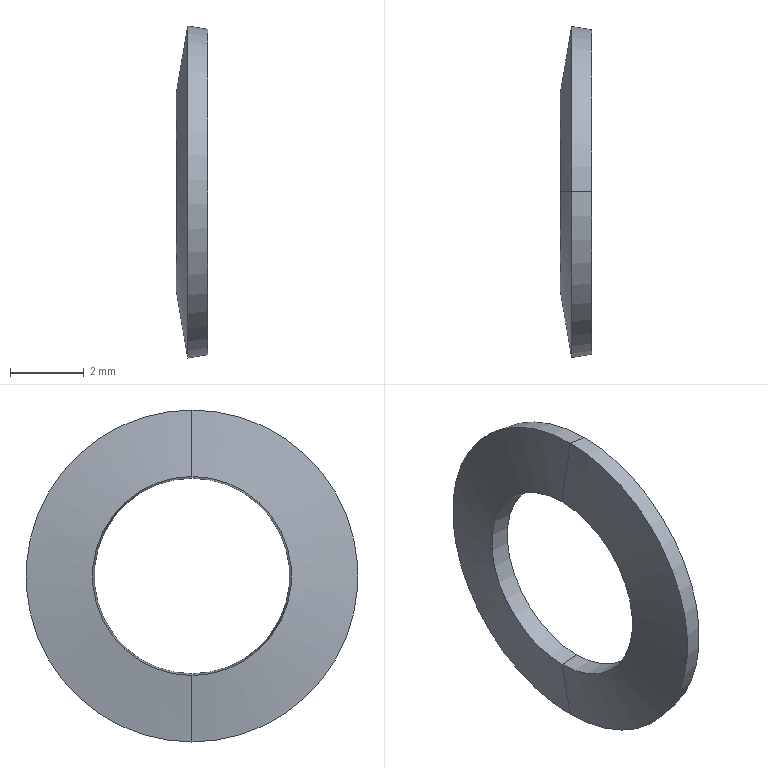Part | STEP file | CW5_Default | 1 solid | 8 faces | box 0.85 x 9 x 9 mm | volume 22.263 mm3 | cone 8
STEP:
#1=CARTESIAN_POINT('',(0.,0.,0.));
#2=DIRECTION('',(0.,0.,1.));
#3=DIRECTION('',(1.,0.,0.));
#4=AXIS2_PLACEMENT_3D('',#1,#2,#3);
#5=CARTESIAN_POINT('',(0.55,0.,2.65));
#6=VERTEX_POINT('',#5);
#7=CARTESIAN_POINT('',(0.,0.,2.697));
#8=VERTEX_POINT('',#7);
#9=CARTESIAN_POINT('',(0.,0.,2.697));
#10=DIRECTION('',(-0.9964,0.,0.08432));
#11=VECTOR('',#10,1.);
#12=LINE('',#9,#11);
#13=CARTESIAN_POINT('',(0.,0.,0.));
#14=DIRECTION('',(-1.,0.,0.));
#15=DIRECTION('',(0.,0.,1.));
#16=AXIS2_PLACEMENT_3D('',#13,#14,#15);
#17=CONICAL_SURFACE('',#16,2.697,0.08442);
#18=CARTESIAN_POINT('',(6.283,0.));
#19=DIRECTION('',(0.,1.));
#20=VECTOR('',#19,1.);
#21=LINE('',#18,#20);
#22=(GEOMETRIC_REPRESENTATION_CONTEXT(2)PARAMETRIC_REPRESENTATION_CONTEXT()REPRESENTATION_CONTEXT('',''));
#23=DEFINITIONAL_REPRESENTATION('',(#21),#22);
#24=PCURVE('',#17,#23);
#25=CARTESIAN_POINT('',(0.,0.,0.));
#26=DIRECTION('',(-1.,0.,0.));
#27=DIRECTION('',(0.,0.,1.));
#28=AXIS2_PLACEMENT_3D('',#25,#26,#27);
#29=CONICAL_SURFACE('',#28,2.697,0.08442);
#30=CARTESIAN_POINT('',(0.,0.));
#31=DIRECTION('',(0.,1.));
#32=VECTOR('',#31,1.);
#33=LINE('',#30,#32);
#34=(GEOMETRIC_REPRESENTATION_CONTEXT(2)PARAMETRIC_REPRESENTATION_CONTEXT()REPRESENTATION_CONTEXT('',''));
#35=DEFINITIONAL_REPRESENTATION('',(#33),#34);
#36=PCURVE('',#29,#35);
#37=SURFACE_CURVE('',#12,(#24,#36),.PCURVE_S1.);
#38=EDGE_CURVE('',#6,#8,#37,.T.);
#39=ORIENTED_EDGE('',*,*,#38,.T.);
#40=CARTESIAN_POINT('',(0.,0.,-2.697));
#41=VERTEX_POINT('',#40);
#42=CARTESIAN_POINT('',(0.,0.,0.));
#43=DIRECTION('',(-1.,0.,0.));
#44=DIRECTION('',(0.,0.,1.));
#45=AXIS2_PLACEMENT_3D('',#42,#43,#44);
#46=CIRCLE('',#45,2.697);
#47=CARTESIAN_POINT('',(0.,0.));
#48=DIRECTION('',(1.,0.));
#49=VECTOR('',#48,1.);
#50=LINE('',#47,#49);
#51=(GEOMETRIC_REPRESENTATION_CONTEXT(2)PARAMETRIC_REPRESENTATION_CONTEXT()REPRESENTATION_CONTEXT('',''));
#52=DEFINITIONAL_REPRESENTATION('',(#50),#51);
#53=PCURVE('',#17,#52);
#54=CARTESIAN_POINT('',(0.3074,0.,0.));
#55=DIRECTION('',(1.,0.,0.));
#56=DIRECTION('',(0.,0.,-1.));
#57=AXIS2_PLACEMENT_3D('',#54,#55,#56);
#58=CONICAL_SURFACE('',#57,4.5,1.402);
#59=CARTESIAN_POINT('',(9.425,-0.3074));
#60=DIRECTION('',(-1.,0.));
#61=VECTOR('',#60,1.);
#62=LINE('',#59,#61);
#63=(GEOMETRIC_REPRESENTATION_CONTEXT(2)PARAMETRIC_REPRESENTATION_CONTEXT()REPRESENTATION_CONTEXT('',''));
#64=DEFINITIONAL_REPRESENTATION('',(#62),#63);
#65=PCURVE('',#58,#64);
#66=SURFACE_CURVE('',#46,(#53,#65),.PCURVE_S1.);
#67=EDGE_CURVE('',#41,#8,#66,.T.);
#68=ORIENTED_EDGE('',*,*,#67,.F.);
#69=CARTESIAN_POINT('',(0.55,0.,-2.65));
#70=VERTEX_POINT('',#69);
#71=CARTESIAN_POINT('',(0.,0.,-2.697));
#72=DIRECTION('',(-0.9964,0.,-0.08432));
#73=VECTOR('',#72,1.);
#74=LINE('',#71,#73);
#75=CARTESIAN_POINT('',(3.142,0.));
#76=DIRECTION('',(0.,1.));
#77=VECTOR('',#76,1.);
#78=LINE('',#75,#77);
#79=(GEOMETRIC_REPRESENTATION_CONTEXT(2)PARAMETRIC_REPRESENTATION_CONTEXT()REPRESENTATION_CONTEXT('',''));
#80=DEFINITIONAL_REPRESENTATION('',(#78),#79);
#81=PCURVE('',#17,#80);
#82=CARTESIAN_POINT('',(3.142,0.));
#83=DIRECTION('',(0.,1.));
#84=VECTOR('',#83,1.);
#85=LINE('',#82,#84);
#86=(GEOMETRIC_REPRESENTATION_CONTEXT(2)PARAMETRIC_REPRESENTATION_CONTEXT()REPRESENTATION_CONTEXT('',''));
#87=DEFINITIONAL_REPRESENTATION('',(#85),#86);
#88=PCURVE('',#29,#87);
#89=SURFACE_CURVE('',#74,(#81,#88),.PCURVE_S1.);
#90=EDGE_CURVE('',#70,#41,#89,.T.);
#91=ORIENTED_EDGE('',*,*,#90,.F.);
#92=CARTESIAN_POINT('',(0.55,0.,0.));
#93=DIRECTION('',(-1.,0.,0.));
#94=DIRECTION('',(0.,0.,1.));
#95=AXIS2_PLACEMENT_3D('',#92,#93,#94);
#96=CIRCLE('',#95,2.65);
#97=CARTESIAN_POINT('',(0.,-0.55));
#98=DIRECTION('',(1.,0.));
#99=VECTOR('',#98,1.);
#100=LINE('',#97,#99);
#101=(GEOMETRIC_REPRESENTATION_CONTEXT(2)PARAMETRIC_REPRESENTATION_CONTEXT()REPRESENTATION_CONTEXT('',''));
#102=DEFINITIONAL_REPRESENTATION('',(#100),#101);
#103=PCURVE('',#17,#102);
#104=CARTESIAN_POINT('',(0.55,0.,0.));
#105=DIRECTION('',(1.,0.,0.));
#106=DIRECTION('',(0.,0.,-1.));
#107=AXIS2_PLACEMENT_3D('',#104,#105,#106);
#108=CONICAL_SURFACE('',#107,2.65,1.402);
#109=CARTESIAN_POINT('',(9.425,0.));
#110=DIRECTION('',(-1.,0.));
#111=VECTOR('',#110,1.);
#112=LINE('',#109,#111);
#113=(GEOMETRIC_REPRESENTATION_CONTEXT(2)PARAMETRIC_REPRESENTATION_CONTEXT()REPRESENTATION_CONTEXT('',''));
#114=DEFINITIONAL_REPRESENTATION('',(#112),#113);
#115=PCURVE('',#108,#114);
#116=SURFACE_CURVE('',#96,(#103,#115),.PCURVE_S1.);
#117=EDGE_CURVE('',#70,#6,#116,.T.);
#118=ORIENTED_EDGE('',*,*,#117,.T.);
#119=EDGE_LOOP('',(#39,#68,#91,#118));
#120=FACE_BOUND('',#119,.F.);
#121=ADVANCED_FACE('',(#120),#17,.F.);
#122=CARTESIAN_POINT('',(0.85,0.,-4.41));
#123=VERTEX_POINT('',#122);
#124=CARTESIAN_POINT('',(0.55,0.,-2.65));
#125=DIRECTION('',(0.168,0.,-0.9858));
#126=VECTOR('',#125,1.);
#127=LINE('',#124,#126);
#128=CARTESIAN_POINT('',(6.283,0.));
#129=DIRECTION('',(0.,1.));
#130=VECTOR('',#129,1.);
#131=LINE('',#128,#130);
#132=(GEOMETRIC_REPRESENTATION_CONTEXT(2)PARAMETRIC_REPRESENTATION_CONTEXT()REPRESENTATION_CONTEXT('',''));
#133=DEFINITIONAL_REPRESENTATION('',(#131),#132);
#134=PCURVE('',#108,#133);
#135=CARTESIAN_POINT('',(0.55,0.,0.));
#136=DIRECTION('',(1.,0.,0.));
#137=DIRECTION('',(0.,0.,-1.));
#138=AXIS2_PLACEMENT_3D('',#135,#136,#137);
#139=CONICAL_SURFACE('',#138,2.65,1.402);
#140=CARTESIAN_POINT('',(0.,0.));
#141=DIRECTION('',(0.,1.));
#142=VECTOR('',#141,1.);
#143=LINE('',#140,#142);
#144=(GEOMETRIC_REPRESENTATION_CONTEXT(2)PARAMETRIC_REPRESENTATION_CONTEXT()REPRESENTATION_CONTEXT('',''));
#145=DEFINITIONAL_REPRESENTATION('',(#143),#144);
#146=PCURVE('',#139,#145);
#147=SURFACE_CURVE('',#127,(#134,#146),.PCURVE_S1.);
#148=EDGE_CURVE('',#70,#123,#147,.T.);
#149=ORIENTED_EDGE('',*,*,#148,.T.);
#150=CARTESIAN_POINT('',(0.85,0.,4.41));
#151=VERTEX_POINT('',#150);
#152=CARTESIAN_POINT('',(0.85,0.,0.));
#153=DIRECTION('',(-1.,0.,0.));
#154=DIRECTION('',(0.,0.,1.));
#155=AXIS2_PLACEMENT_3D('',#152,#153,#154);
#156=CIRCLE('',#155,4.41);
#157=CARTESIAN_POINT('',(9.425,0.3));
#158=DIRECTION('',(-1.,0.));
#159=VECTOR('',#158,1.);
#160=LINE('',#157,#159);
#161=(GEOMETRIC_REPRESENTATION_CONTEXT(2)PARAMETRIC_REPRESENTATION_CONTEXT()REPRESENTATION_CONTEXT('',''));
#162=DEFINITIONAL_REPRESENTATION('',(#160),#161);
#163=PCURVE('',#108,#162);
#164=CARTESIAN_POINT('',(0.85,0.,0.));
#165=DIRECTION('',(-1.,0.,0.));
#166=DIRECTION('',(0.,0.,1.));
#167=AXIS2_PLACEMENT_3D('',#164,#165,#166);
#168=CONICAL_SURFACE('',#167,4.41,0.1644);
#169=CARTESIAN_POINT('',(0.,0.));
#170=DIRECTION('',(1.,0.));
#171=VECTOR('',#170,1.);
#172=LINE('',#169,#171);
#173=(GEOMETRIC_REPRESENTATION_CONTEXT(2)PARAMETRIC_REPRESENTATION_CONTEXT()REPRESENTATION_CONTEXT('',''));
#174=DEFINITIONAL_REPRESENTATION('',(#172),#173);
#175=PCURVE('',#168,#174);
#176=SURFACE_CURVE('',#156,(#163,#175),.PCURVE_S1.);
#177=EDGE_CURVE('',#123,#151,#176,.T.);
#178=ORIENTED_EDGE('',*,*,#177,.T.);
#179=CARTESIAN_POINT('',(0.55,0.,2.65));
#180=DIRECTION('',(0.168,0.,0.9858));
#181=VECTOR('',#180,1.);
#182=LINE('',#179,#181);
#183=CARTESIAN_POINT('',(3.142,0.));
#184=DIRECTION('',(0.,1.));
#185=VECTOR('',#184,1.);
#186=LINE('',#183,#185);
#187=(GEOMETRIC_REPRESENTATION_CONTEXT(2)PARAMETRIC_REPRESENTATION_CONTEXT()REPRESENTATION_CONTEXT('',''));
#188=DEFINITIONAL_REPRESENTATION('',(#186),#187);
#189=PCURVE('',#108,#188);
#190=CARTESIAN_POINT('',(3.142,0.));
#191=DIRECTION('',(0.,1.));
#192=VECTOR('',#191,1.);
#193=LINE('',#190,#192);
#194=(GEOMETRIC_REPRESENTATION_CONTEXT(2)PARAMETRIC_REPRESENTATION_CONTEXT()REPRESENTATION_CONTEXT('',''));
#195=DEFINITIONAL_REPRESENTATION('',(#193),#194);
#196=PCURVE('',#139,#195);
#197=SURFACE_CURVE('',#182,(#189,#196),.PCURVE_S1.);
#198=EDGE_CURVE('',#6,#151,#197,.T.);
#199=ORIENTED_EDGE('',*,*,#198,.F.);
#200=ORIENTED_EDGE('',*,*,#117,.F.);
#201=EDGE_LOOP('',(#149,#178,#199,#200));
#202=FACE_BOUND('',#201,.F.);
#203=ADVANCED_FACE('',(#202),#108,.F.);
#204=CARTESIAN_POINT('',(0.85,0.,0.));
#205=DIRECTION('',(-1.,0.,0.));
#206=DIRECTION('',(0.,0.,1.));
#207=AXIS2_PLACEMENT_3D('',#204,#205,#206);
#208=CIRCLE('',#207,4.41);
#209=CARTESIAN_POINT('',(0.85,0.,0.));
#210=DIRECTION('',(-1.,0.,0.));
#211=DIRECTION('',(0.,0.,1.));
#212=AXIS2_PLACEMENT_3D('',#209,#210,#211);
#213=CONICAL_SURFACE('',#212,4.41,0.1644);
#214=CARTESIAN_POINT('',(0.,0.));
#215=DIRECTION('',(1.,0.));
#216=VECTOR('',#215,1.);
#217=LINE('',#214,#216);
#218=(GEOMETRIC_REPRESENTATION_CONTEXT(2)PARAMETRIC_REPRESENTATION_CONTEXT()REPRESENTATION_CONTEXT('',''));
#219=DEFINITIONAL_REPRESENTATION('',(#217),#218);
#220=PCURVE('',#213,#219);
#221=CARTESIAN_POINT('',(3.142,0.3));
#222=DIRECTION('',(-1.,0.));
#223=VECTOR('',#222,1.);
#224=LINE('',#221,#223);
#225=(GEOMETRIC_REPRESENTATION_CONTEXT(2)PARAMETRIC_REPRESENTATION_CONTEXT()REPRESENTATION_CONTEXT('',''));
#226=DEFINITIONAL_REPRESENTATION('',(#224),#225);
#227=PCURVE('',#139,#226);
#228=SURFACE_CURVE('',#208,(#220,#227),.PCURVE_S1.);
#229=EDGE_CURVE('',#151,#123,#228,.T.);
#230=ORIENTED_EDGE('',*,*,#229,.T.);
#231=CARTESIAN_POINT('',(0.3074,0.,-4.5));
#232=VERTEX_POINT('',#231);
#233=CARTESIAN_POINT('',(0.85,0.,-4.41));
#234=DIRECTION('',(-0.9865,0.,-0.1636));
#235=VECTOR('',#234,1.);
#236=LINE('',#233,#235);
#237=CARTESIAN_POINT('',(3.142,0.));
#238=DIRECTION('',(0.,1.));
#239=VECTOR('',#238,1.);
#240=LINE('',#237,#239);
#241=(GEOMETRIC_REPRESENTATION_CONTEXT(2)PARAMETRIC_REPRESENTATION_CONTEXT()REPRESENTATION_CONTEXT('',''));
#242=DEFINITIONAL_REPRESENTATION('',(#240),#241);
#243=PCURVE('',#213,#242);
#244=CARTESIAN_POINT('',(3.142,0.));
#245=DIRECTION('',(0.,1.));
#246=VECTOR('',#245,1.);
#247=LINE('',#244,#246);
#248=(GEOMETRIC_REPRESENTATION_CONTEXT(2)PARAMETRIC_REPRESENTATION_CONTEXT()REPRESENTATION_CONTEXT('',''));
#249=DEFINITIONAL_REPRESENTATION('',(#247),#248);
#250=PCURVE('',#168,#249);
#251=SURFACE_CURVE('',#236,(#243,#250),.PCURVE_S1.);
#252=EDGE_CURVE('',#123,#232,#251,.T.);
#253=ORIENTED_EDGE('',*,*,#252,.T.);
#254=CARTESIAN_POINT('',(0.3074,0.,4.5));
#255=VERTEX_POINT('',#254);
#256=CARTESIAN_POINT('',(0.3074,0.,0.));
#257=DIRECTION('',(-1.,0.,0.));
#258=DIRECTION('',(0.,0.,1.));
#259=AXIS2_PLACEMENT_3D('',#256,#257,#258);
#260=CIRCLE('',#259,4.5);
#261=CARTESIAN_POINT('',(0.,0.5426));
#262=DIRECTION('',(1.,0.));
#263=VECTOR('',#262,1.);
#264=LINE('',#261,#263);
#265=(GEOMETRIC_REPRESENTATION_CONTEXT(2)PARAMETRIC_REPRESENTATION_CONTEXT()REPRESENTATION_CONTEXT('',''));
#266=DEFINITIONAL_REPRESENTATION('',(#264),#265);
#267=PCURVE('',#213,#266);
#268=CARTESIAN_POINT('',(0.3074,0.,0.));
#269=DIRECTION('',(1.,0.,0.));
#270=DIRECTION('',(0.,0.,-1.));
#271=AXIS2_PLACEMENT_3D('',#268,#269,#270);
#272=CONICAL_SURFACE('',#271,4.5,1.402);
#273=CARTESIAN_POINT('',(3.142,0.));
#274=DIRECTION('',(-1.,0.));
#275=VECTOR('',#274,1.);
#276=LINE('',#273,#275);
#277=(GEOMETRIC_REPRESENTATION_CONTEXT(2)PARAMETRIC_REPRESENTATION_CONTEXT()REPRESENTATION_CONTEXT('',''));
#278=DEFINITIONAL_REPRESENTATION('',(#276),#277);
#279=PCURVE('',#272,#278);
#280=SURFACE_CURVE('',#260,(#267,#279),.PCURVE_S1.);
#281=EDGE_CURVE('',#255,#232,#280,.T.);
#282=ORIENTED_EDGE('',*,*,#281,.F.);
#283=CARTESIAN_POINT('',(0.85,0.,4.41));
#284=DIRECTION('',(-0.9865,0.,0.1636));
#285=VECTOR('',#284,1.);
#286=LINE('',#283,#285);
#287=CARTESIAN_POINT('',(0.,0.));
#288=DIRECTION('',(0.,1.));
#289=VECTOR('',#288,1.);
#290=LINE('',#287,#289);
#291=(GEOMETRIC_REPRESENTATION_CONTEXT(2)PARAMETRIC_REPRESENTATION_CONTEXT()REPRESENTATION_CONTEXT('',''));
#292=DEFINITIONAL_REPRESENTATION('',(#290),#291);
#293=PCURVE('',#213,#292);
#294=CARTESIAN_POINT('',(6.283,0.));
#295=DIRECTION('',(0.,1.));
#296=VECTOR('',#295,1.);
#297=LINE('',#294,#296);
#298=(GEOMETRIC_REPRESENTATION_CONTEXT(2)PARAMETRIC_REPRESENTATION_CONTEXT()REPRESENTATION_CONTEXT('',''));
#299=DEFINITIONAL_REPRESENTATION('',(#297),#298);
#300=PCURVE('',#168,#299);
#301=SURFACE_CURVE('',#286,(#293,#300),.PCURVE_S1.);
#302=EDGE_CURVE('',#151,#255,#301,.T.);
#303=ORIENTED_EDGE('',*,*,#302,.F.);
#304=EDGE_LOOP('',(#230,#253,#282,#303));
#305=FACE_BOUND('',#304,.T.);
#306=ADVANCED_FACE('',(#305),#213,.T.);
#307=CARTESIAN_POINT('',(0.,0.,0.));
#308=DIRECTION('',(-1.,0.,0.));
#309=DIRECTION('',(0.,0.,1.));
#310=AXIS2_PLACEMENT_3D('',#307,#308,#309);
#311=CIRCLE('',#310,2.697);
#312=CARTESIAN_POINT('',(3.142,-0.3074));
#313=DIRECTION('',(-1.,0.));
#314=VECTOR('',#313,1.);
#315=LINE('',#312,#314);
#316=(GEOMETRIC_REPRESENTATION_CONTEXT(2)PARAMETRIC_REPRESENTATION_CONTEXT()REPRESENTATION_CONTEXT('',''));
#317=DEFINITIONAL_REPRESENTATION('',(#315),#316);
#318=PCURVE('',#272,#317);
#319=CARTESIAN_POINT('',(0.,0.));
#320=DIRECTION('',(1.,0.));
#321=VECTOR('',#320,1.);
#322=LINE('',#319,#321);
#323=(GEOMETRIC_REPRESENTATION_CONTEXT(2)PARAMETRIC_REPRESENTATION_CONTEXT()REPRESENTATION_CONTEXT('',''));
#324=DEFINITIONAL_REPRESENTATION('',(#322),#323);
#325=PCURVE('',#29,#324);
#326=SURFACE_CURVE('',#311,(#318,#325),.PCURVE_S1.);
#327=EDGE_CURVE('',#8,#41,#326,.T.);
#328=ORIENTED_EDGE('',*,*,#327,.F.);
#329=CARTESIAN_POINT('',(0.3074,0.,4.5));
#330=DIRECTION('',(0.168,0.,0.9858));
#331=VECTOR('',#330,1.);
#332=LINE('',#329,#331);
#333=CARTESIAN_POINT('',(3.142,0.));
#334=DIRECTION('',(0.,1.));
#335=VECTOR('',#334,1.);
#336=LINE('',#333,#335);
#337=(GEOMETRIC_REPRESENTATION_CONTEXT(2)PARAMETRIC_REPRESENTATION_CONTEXT()REPRESENTATION_CONTEXT('',''));
#338=DEFINITIONAL_REPRESENTATION('',(#336),#337);
#339=PCURVE('',#272,#338);
#340=CARTESIAN_POINT('',(3.142,0.));
#341=DIRECTION('',(0.,1.));
#342=VECTOR('',#341,1.);
#343=LINE('',#340,#342);
#344=(GEOMETRIC_REPRESENTATION_CONTEXT(2)PARAMETRIC_REPRESENTATION_CONTEXT()REPRESENTATION_CONTEXT('',''));
#345=DEFINITIONAL_REPRESENTATION('',(#343),#344);
#346=PCURVE('',#58,#345);
#347=SURFACE_CURVE('',#332,(#339,#346),.PCURVE_S1.);
#348=EDGE_CURVE('',#8,#255,#347,.T.);
#349=ORIENTED_EDGE('',*,*,#348,.T.);
#350=ORIENTED_EDGE('',*,*,#281,.T.);
#351=CARTESIAN_POINT('',(0.3074,0.,-4.5));
#352=DIRECTION('',(0.168,0.,-0.9858));
#353=VECTOR('',#352,1.);
#354=LINE('',#351,#353);
#355=CARTESIAN_POINT('',(0.,0.));
#356=DIRECTION('',(0.,1.));
#357=VECTOR('',#356,1.);
#358=LINE('',#355,#357);
#359=(GEOMETRIC_REPRESENTATION_CONTEXT(2)PARAMETRIC_REPRESENTATION_CONTEXT()REPRESENTATION_CONTEXT('',''));
#360=DEFINITIONAL_REPRESENTATION('',(#358),#359);
#361=PCURVE('',#272,#360);
#362=CARTESIAN_POINT('',(6.283,0.));
#363=DIRECTION('',(0.,1.));
#364=VECTOR('',#363,1.);
#365=LINE('',#362,#364);
#366=(GEOMETRIC_REPRESENTATION_CONTEXT(2)PARAMETRIC_REPRESENTATION_CONTEXT()REPRESENTATION_CONTEXT('',''));
#367=DEFINITIONAL_REPRESENTATION('',(#365),#366);
#368=PCURVE('',#58,#367);
#369=SURFACE_CURVE('',#354,(#361,#368),.PCURVE_S1.);
#370=EDGE_CURVE('',#41,#232,#369,.T.);
#371=ORIENTED_EDGE('',*,*,#370,.F.);
#372=EDGE_LOOP('',(#328,#349,#350,#371));
#373=FACE_BOUND('',#372,.T.);
#374=ADVANCED_FACE('',(#373),#272,.T.);
#375=ORIENTED_EDGE('',*,*,#348,.F.);
#376=ORIENTED_EDGE('',*,*,#67,.F.);
#377=ORIENTED_EDGE('',*,*,#370,.T.);
#378=CARTESIAN_POINT('',(0.3074,0.,0.));
#379=DIRECTION('',(-1.,0.,0.));
#380=DIRECTION('',(0.,0.,1.));
#381=AXIS2_PLACEMENT_3D('',#378,#379,#380);
#382=CIRCLE('',#381,4.5);
#383=CARTESIAN_POINT('',(9.425,0.));
#384=DIRECTION('',(-1.,0.));
#385=VECTOR('',#384,1.);
#386=LINE('',#383,#385);
#387=(GEOMETRIC_REPRESENTATION_CONTEXT(2)PARAMETRIC_REPRESENTATION_CONTEXT()REPRESENTATION_CONTEXT('',''));
#388=DEFINITIONAL_REPRESENTATION('',(#386),#387);
#389=PCURVE('',#58,#388);
#390=CARTESIAN_POINT('',(0.,0.5426));
#391=DIRECTION('',(1.,0.));
#392=VECTOR('',#391,1.);
#393=LINE('',#390,#392);
#394=(GEOMETRIC_REPRESENTATION_CONTEXT(2)PARAMETRIC_REPRESENTATION_CONTEXT()REPRESENTATION_CONTEXT('',''));
#395=DEFINITIONAL_REPRESENTATION('',(#393),#394);
#396=PCURVE('',#168,#395);
#397=SURFACE_CURVE('',#382,(#389,#396),.PCURVE_S1.);
#398=EDGE_CURVE('',#232,#255,#397,.T.);
#399=ORIENTED_EDGE('',*,*,#398,.T.);
#400=EDGE_LOOP('',(#375,#376,#377,#399));
#401=FACE_BOUND('',#400,.T.);
#402=ADVANCED_FACE('',(#401),#58,.T.);
#403=ORIENTED_EDGE('',*,*,#252,.F.);
#404=ORIENTED_EDGE('',*,*,#177,.T.);
#405=ORIENTED_EDGE('',*,*,#302,.T.);
#406=ORIENTED_EDGE('',*,*,#398,.F.);
#407=EDGE_LOOP('',(#403,#404,#405,#406));
#408=FACE_BOUND('',#407,.T.);
#409=ADVANCED_FACE('',(#408),#168,.T.);
#410=ORIENTED_EDGE('',*,*,#229,.T.);
#411=ORIENTED_EDGE('',*,*,#148,.F.);
#412=CARTESIAN_POINT('',(0.55,0.,0.));
#413=DIRECTION('',(-1.,0.,0.));
#414=DIRECTION('',(0.,0.,1.));
#415=AXIS2_PLACEMENT_3D('',#412,#413,#414);
#416=CIRCLE('',#415,2.65);
#417=CARTESIAN_POINT('',(3.142,0.));
#418=DIRECTION('',(-1.,0.));
#419=VECTOR('',#418,1.);
#420=LINE('',#417,#419);
#421=(GEOMETRIC_REPRESENTATION_CONTEXT(2)PARAMETRIC_REPRESENTATION_CONTEXT()REPRESENTATION_CONTEXT('',''));
#422=DEFINITIONAL_REPRESENTATION('',(#420),#421);
#423=PCURVE('',#139,#422);
#424=CARTESIAN_POINT('',(0.,-0.55));
#425=DIRECTION('',(1.,0.));
#426=VECTOR('',#425,1.);
#427=LINE('',#424,#426);
#428=(GEOMETRIC_REPRESENTATION_CONTEXT(2)PARAMETRIC_REPRESENTATION_CONTEXT()REPRESENTATION_CONTEXT('',''));
#429=DEFINITIONAL_REPRESENTATION('',(#427),#428);
#430=PCURVE('',#29,#429);
#431=SURFACE_CURVE('',#416,(#423,#430),.PCURVE_S1.);
#432=EDGE_CURVE('',#6,#70,#431,.T.);
#433=ORIENTED_EDGE('',*,*,#432,.F.);
#434=ORIENTED_EDGE('',*,*,#198,.T.);
#435=EDGE_LOOP('',(#410,#411,#433,#434));
#436=FACE_BOUND('',#435,.F.);
#437=ADVANCED_FACE('',(#436),#139,.F.);
#438=ORIENTED_EDGE('',*,*,#327,.F.);
#439=ORIENTED_EDGE('',*,*,#38,.F.);
#440=ORIENTED_EDGE('',*,*,#432,.T.);
#441=ORIENTED_EDGE('',*,*,#90,.T.);
#442=EDGE_LOOP('',(#438,#439,#440,#441));
#443=FACE_BOUND('',#442,.F.);
#444=ADVANCED_FACE('',(#443),#29,.F.);
#445=CLOSED_SHELL('',(#121,#203,#306,#374,#402,#409,#437,#444));
#446=MANIFOLD_SOLID_BREP('',#445);
#447=(LENGTH_UNIT()NAMED_UNIT(*)SI_UNIT(.MILLI.,.METRE.));
#448=UNCERTAINTY_MEASURE_WITH_UNIT(LENGTH_MEASURE(0.0000001),#447,'','');
#449=(NAMED_UNIT(*)PLANE_ANGLE_UNIT()SI_UNIT($,.RADIAN.));
#450=(NAMED_UNIT(*)SI_UNIT($,.STERADIAN.)SOLID_ANGLE_UNIT());
#451=(GEOMETRIC_REPRESENTATION_CONTEXT(3)GLOBAL_UNCERTAINTY_ASSIGNED_CONTEXT((#448))GLOBAL_UNIT_ASSIGNED_CONTEXT((#447,#449,#450))REPRESENTATION_CONTEXT('',''));
#452=ADVANCED_BREP_SHAPE_REPRESENTATION('',(#4,#446),#451);